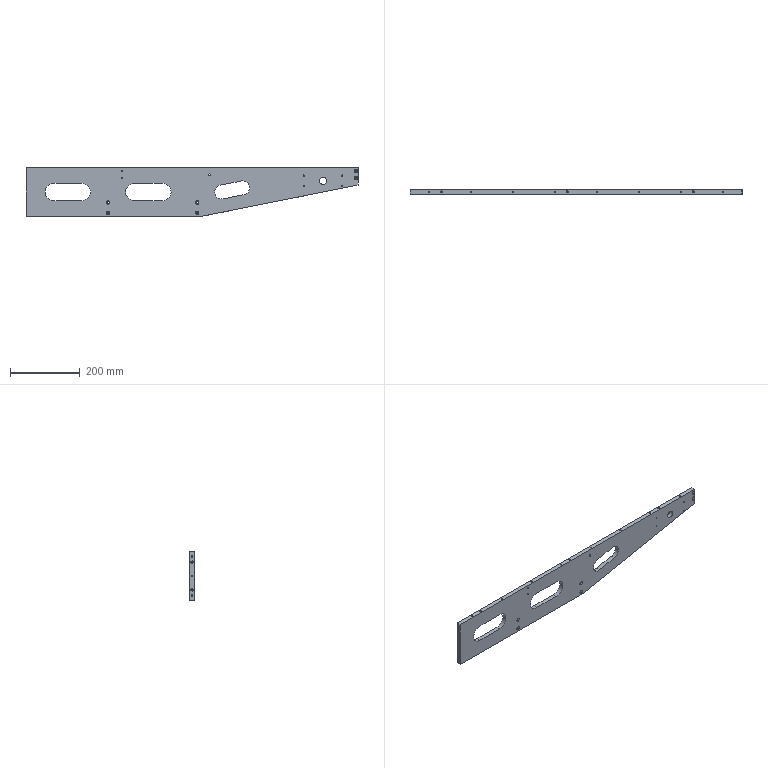Part | SolidWorks | features HoleWzd 10, ICE 2, Chamfer 1 | 1 solid | 167 faces | box 950 x 12 x 140 mm | volume 1151524 mm3 | cylinder 91 | cone 54 | plane 22 | commonest cylinder face diameters 3.3 x20 4.2 x16 5.5 x12 10 x12 5 x10 6 x10